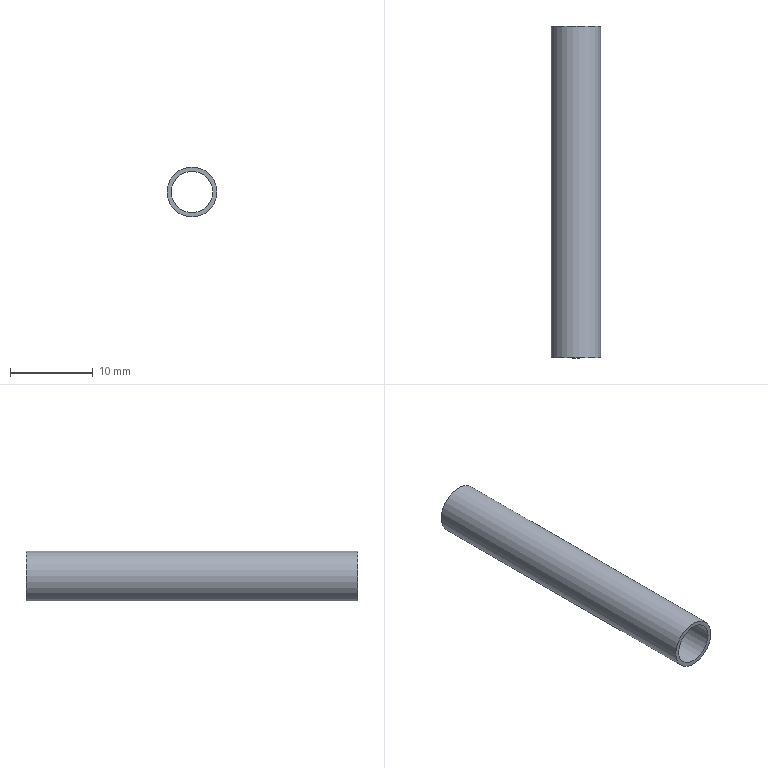Part | STEP file | 1-73.7 | 1 solid | 4 faces | box 6 x 40 x 6 mm | volume 345.575 mm3 | cylinder 2 | plane 2 | commonest cylinder face diameters 5 x1 6 x1
STEP:
#1=CARTESIAN_POINT('',(0.,0.,0.));
#2=DIRECTION('',(0.,0.,1.));
#3=DIRECTION('',(1.,0.,0.));
#4=AXIS2_PLACEMENT_3D('',#1,#2,#3);
#5=CARTESIAN_POINT('',(3.,0.,0.));
#6=VERTEX_POINT('',#5);
#7=CARTESIAN_POINT('',(0.,0.,0.));
#8=DIRECTION('',(0.,-1.,0.));
#9=DIRECTION('',(1.,0.,0.));
#10=AXIS2_PLACEMENT_3D('',#7,#8,#9);
#11=CIRCLE('',#10,3.);
#12=CARTESIAN_POINT('',(0.,0.,0.));
#13=DIRECTION('',(0.,1.,0.));
#14=DIRECTION('',(1.,0.,0.));
#15=AXIS2_PLACEMENT_3D('',#12,#13,#14);
#16=CYLINDRICAL_SURFACE('',#15,3.);
#17=CARTESIAN_POINT('',(6.283,0.));
#18=DIRECTION('',(-1.,0.));
#19=VECTOR('',#18,1.);
#20=LINE('',#17,#19);
#21=(GEOMETRIC_REPRESENTATION_CONTEXT(2)PARAMETRIC_REPRESENTATION_CONTEXT()REPRESENTATION_CONTEXT('',''));
#22=DEFINITIONAL_REPRESENTATION('',(#20),#21);
#23=PCURVE('',#16,#22);
#24=CARTESIAN_POINT('',(0.,0.,0.));
#25=DIRECTION('',(0.,-1.,0.));
#26=DIRECTION('',(1.,0.,0.));
#27=AXIS2_PLACEMENT_3D('',#24,#25,#26);
#28=PLANE('',#27);
#29=CARTESIAN_POINT('',(0.,0.));
#30=DIRECTION('',(1.,0.));
#31=AXIS2_PLACEMENT_2D('',#29,#30);
#32=CIRCLE('',#31,3.);
#33=(GEOMETRIC_REPRESENTATION_CONTEXT(2)PARAMETRIC_REPRESENTATION_CONTEXT()REPRESENTATION_CONTEXT('',''));
#34=DEFINITIONAL_REPRESENTATION('',(#32),#33);
#35=PCURVE('',#28,#34);
#36=SURFACE_CURVE('',#11,(#23,#35),.PCURVE_S1.);
#37=EDGE_CURVE('',#6,#6,#36,.T.);
#38=ORIENTED_EDGE('',*,*,#37,.F.);
#39=CARTESIAN_POINT('',(3.,40.,0.));
#40=VERTEX_POINT('',#39);
#41=CARTESIAN_POINT('',(3.,0.,0.));
#42=DIRECTION('',(0.,1.,0.));
#43=VECTOR('',#42,1.);
#44=LINE('',#41,#43);
#45=CARTESIAN_POINT('',(6.283,0.));
#46=DIRECTION('',(0.,1.));
#47=VECTOR('',#46,1.);
#48=LINE('',#45,#47);
#49=(GEOMETRIC_REPRESENTATION_CONTEXT(2)PARAMETRIC_REPRESENTATION_CONTEXT()REPRESENTATION_CONTEXT('',''));
#50=DEFINITIONAL_REPRESENTATION('',(#48),#49);
#51=PCURVE('',#16,#50);
#52=CARTESIAN_POINT('',(0.,0.));
#53=DIRECTION('',(0.,1.));
#54=VECTOR('',#53,1.);
#55=LINE('',#52,#54);
#56=(GEOMETRIC_REPRESENTATION_CONTEXT(2)PARAMETRIC_REPRESENTATION_CONTEXT()REPRESENTATION_CONTEXT('',''));
#57=DEFINITIONAL_REPRESENTATION('',(#55),#56);
#58=PCURVE('',#16,#57);
#59=SEAM_CURVE('',#44,(#51,#58),.PCURVE_S1.);
#60=EDGE_CURVE('',#6,#40,#59,.T.);
#61=ORIENTED_EDGE('',*,*,#60,.T.);
#62=CARTESIAN_POINT('',(0.,40.,0.));
#63=DIRECTION('',(0.,1.,0.));
#64=DIRECTION('',(1.,0.,0.));
#65=AXIS2_PLACEMENT_3D('',#62,#63,#64);
#66=CIRCLE('',#65,3.);
#67=CARTESIAN_POINT('',(0.,40.));
#68=DIRECTION('',(1.,0.));
#69=VECTOR('',#68,1.);
#70=LINE('',#67,#69);
#71=(GEOMETRIC_REPRESENTATION_CONTEXT(2)PARAMETRIC_REPRESENTATION_CONTEXT()REPRESENTATION_CONTEXT('',''));
#72=DEFINITIONAL_REPRESENTATION('',(#70),#71);
#73=PCURVE('',#16,#72);
#74=CARTESIAN_POINT('',(0.,40.,0.));
#75=DIRECTION('',(0.,1.,0.));
#76=DIRECTION('',(0.,0.,1.));
#77=AXIS2_PLACEMENT_3D('',#74,#75,#76);
#78=PLANE('',#77);
#79=CARTESIAN_POINT('',(0.,0.));
#80=DIRECTION('',(0.,1.));
#81=AXIS2_PLACEMENT_2D('',#79,#80);
#82=CIRCLE('',#81,3.);
#83=(GEOMETRIC_REPRESENTATION_CONTEXT(2)PARAMETRIC_REPRESENTATION_CONTEXT()REPRESENTATION_CONTEXT('',''));
#84=DEFINITIONAL_REPRESENTATION('',(#82),#83);
#85=PCURVE('',#78,#84);
#86=SURFACE_CURVE('',#66,(#73,#85),.PCURVE_S1.);
#87=EDGE_CURVE('',#40,#40,#86,.T.);
#88=ORIENTED_EDGE('',*,*,#87,.F.);
#89=ORIENTED_EDGE('',*,*,#60,.F.);
#90=EDGE_LOOP('',(#38,#61,#88,#89));
#91=FACE_BOUND('',#90,.T.);
#92=ADVANCED_FACE('',(#91),#16,.T.);
#93=ORIENTED_EDGE('',*,*,#37,.T.);
#94=EDGE_LOOP('',(#93));
#95=FACE_BOUND('',#94,.T.);
#96=CARTESIAN_POINT('',(2.5,0.,0.));
#97=VERTEX_POINT('',#96);
#98=CARTESIAN_POINT('',(0.,0.,0.));
#99=DIRECTION('',(0.,-1.,0.));
#100=DIRECTION('',(1.,0.,0.));
#101=AXIS2_PLACEMENT_3D('',#98,#99,#100);
#102=CIRCLE('',#101,2.5);
#103=CARTESIAN_POINT('',(0.,0.));
#104=DIRECTION('',(1.,0.));
#105=AXIS2_PLACEMENT_2D('',#103,#104);
#106=CIRCLE('',#105,2.5);
#107=(GEOMETRIC_REPRESENTATION_CONTEXT(2)PARAMETRIC_REPRESENTATION_CONTEXT()REPRESENTATION_CONTEXT('',''));
#108=DEFINITIONAL_REPRESENTATION('',(#106),#107);
#109=PCURVE('',#28,#108);
#110=CARTESIAN_POINT('',(0.,0.,0.));
#111=DIRECTION('',(0.,1.,0.));
#112=DIRECTION('',(1.,0.,0.));
#113=AXIS2_PLACEMENT_3D('',#110,#111,#112);
#114=CYLINDRICAL_SURFACE('',#113,2.5);
#115=CARTESIAN_POINT('',(6.283,0.));
#116=DIRECTION('',(-1.,0.));
#117=VECTOR('',#116,1.);
#118=LINE('',#115,#117);
#119=(GEOMETRIC_REPRESENTATION_CONTEXT(2)PARAMETRIC_REPRESENTATION_CONTEXT()REPRESENTATION_CONTEXT('',''));
#120=DEFINITIONAL_REPRESENTATION('',(#118),#119);
#121=PCURVE('',#114,#120);
#122=SURFACE_CURVE('',#102,(#109,#121),.PCURVE_S1.);
#123=EDGE_CURVE('',#97,#97,#122,.T.);
#124=ORIENTED_EDGE('',*,*,#123,.F.);
#125=EDGE_LOOP('',(#124));
#126=FACE_BOUND('',#125,.T.);
#127=ADVANCED_FACE('',(#95,#126),#28,.T.);
#128=ORIENTED_EDGE('',*,*,#87,.T.);
#129=EDGE_LOOP('',(#128));
#130=FACE_BOUND('',#129,.T.);
#131=CARTESIAN_POINT('',(2.5,40.,0.));
#132=VERTEX_POINT('',#131);
#133=CARTESIAN_POINT('',(0.,40.,0.));
#134=DIRECTION('',(0.,1.,0.));
#135=DIRECTION('',(1.,0.,0.));
#136=AXIS2_PLACEMENT_3D('',#133,#134,#135);
#137=CIRCLE('',#136,2.5);
#138=CARTESIAN_POINT('',(0.,0.));
#139=DIRECTION('',(0.,1.));
#140=AXIS2_PLACEMENT_2D('',#138,#139);
#141=CIRCLE('',#140,2.5);
#142=(GEOMETRIC_REPRESENTATION_CONTEXT(2)PARAMETRIC_REPRESENTATION_CONTEXT()REPRESENTATION_CONTEXT('',''));
#143=DEFINITIONAL_REPRESENTATION('',(#141),#142);
#144=PCURVE('',#78,#143);
#145=CARTESIAN_POINT('',(0.,40.));
#146=DIRECTION('',(1.,0.));
#147=VECTOR('',#146,1.);
#148=LINE('',#145,#147);
#149=(GEOMETRIC_REPRESENTATION_CONTEXT(2)PARAMETRIC_REPRESENTATION_CONTEXT()REPRESENTATION_CONTEXT('',''));
#150=DEFINITIONAL_REPRESENTATION('',(#148),#149);
#151=PCURVE('',#114,#150);
#152=SURFACE_CURVE('',#137,(#144,#151),.PCURVE_S1.);
#153=EDGE_CURVE('',#132,#132,#152,.T.);
#154=ORIENTED_EDGE('',*,*,#153,.F.);
#155=EDGE_LOOP('',(#154));
#156=FACE_BOUND('',#155,.T.);
#157=ADVANCED_FACE('',(#130,#156),#78,.T.);
#158=ORIENTED_EDGE('',*,*,#123,.F.);
#159=CARTESIAN_POINT('',(2.5,0.,0.));
#160=DIRECTION('',(0.,1.,0.));
#161=VECTOR('',#160,1.);
#162=LINE('',#159,#161);
#163=CARTESIAN_POINT('',(6.283,0.));
#164=DIRECTION('',(0.,1.));
#165=VECTOR('',#164,1.);
#166=LINE('',#163,#165);
#167=(GEOMETRIC_REPRESENTATION_CONTEXT(2)PARAMETRIC_REPRESENTATION_CONTEXT()REPRESENTATION_CONTEXT('',''));
#168=DEFINITIONAL_REPRESENTATION('',(#166),#167);
#169=PCURVE('',#114,#168);
#170=CARTESIAN_POINT('',(0.,0.));
#171=DIRECTION('',(0.,1.));
#172=VECTOR('',#171,1.);
#173=LINE('',#170,#172);
#174=(GEOMETRIC_REPRESENTATION_CONTEXT(2)PARAMETRIC_REPRESENTATION_CONTEXT()REPRESENTATION_CONTEXT('',''));
#175=DEFINITIONAL_REPRESENTATION('',(#173),#174);
#176=PCURVE('',#114,#175);
#177=SEAM_CURVE('',#162,(#169,#176),.PCURVE_S1.);
#178=EDGE_CURVE('',#97,#132,#177,.T.);
#179=ORIENTED_EDGE('',*,*,#178,.T.);
#180=ORIENTED_EDGE('',*,*,#153,.F.);
#181=ORIENTED_EDGE('',*,*,#178,.F.);
#182=EDGE_LOOP('',(#158,#179,#180,#181));
#183=FACE_BOUND('',#182,.F.);
#184=ADVANCED_FACE('',(#183),#114,.F.);
#185=CLOSED_SHELL('',(#92,#127,#157,#184));
#186=MANIFOLD_SOLID_BREP('',#185);
#187=(LENGTH_UNIT()NAMED_UNIT(*)SI_UNIT(.MILLI.,.METRE.));
#188=UNCERTAINTY_MEASURE_WITH_UNIT(LENGTH_MEASURE(0.0000001),#187,'','');
#189=(NAMED_UNIT(*)PLANE_ANGLE_UNIT()SI_UNIT($,.RADIAN.));
#190=(NAMED_UNIT(*)SI_UNIT($,.STERADIAN.)SOLID_ANGLE_UNIT());
#191=(GEOMETRIC_REPRESENTATION_CONTEXT(3)GLOBAL_UNCERTAINTY_ASSIGNED_CONTEXT((#188))GLOBAL_UNIT_ASSIGNED_CONTEXT((#187,#189,#190))REPRESENTATION_CONTEXT('',''));
#192=ADVANCED_BREP_SHAPE_REPRESENTATION('',(#4,#186),#191);